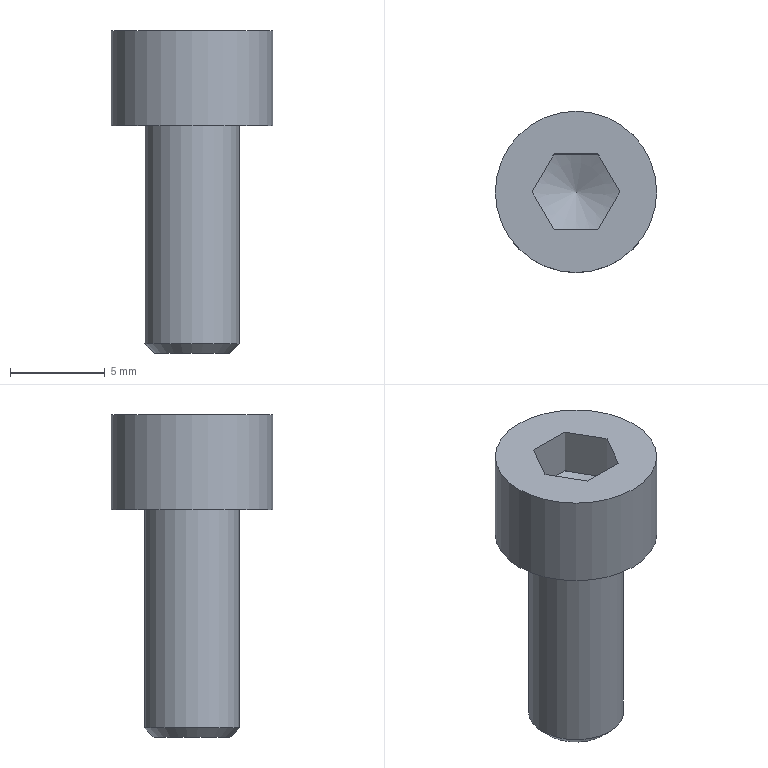Part | STEP file | 3_id510_xmt_txt | 1 solid | 25 faces | box 8.5 x 8.5 x 17 mm | volume 477.285 mm3 | plane 21 | cylinder 2 | cone 2 | commonest cylinder face diameters 5 x1 8.5 x1